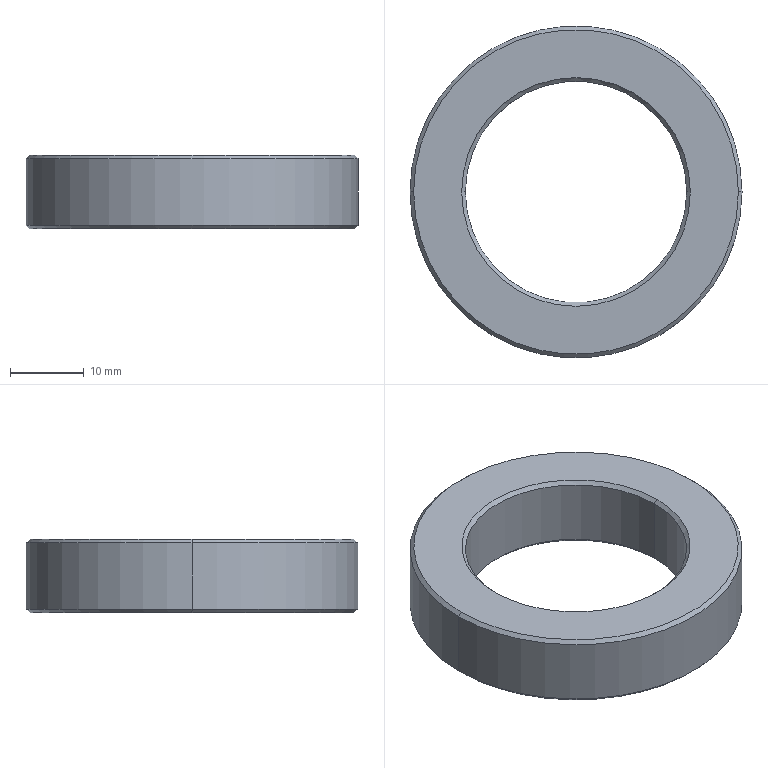Part | SolidWorks | features Chamfer 1, Extrusion 1 | 1 solid | 14 faces | box 45 x 45 x 10 mm | volume 8777 mm3 | cone 8 | cylinder 4 | plane 2 | commonest cylinder face diameters 30 x2 45 x2
STEP:
#1=CARTESIAN_POINT('',(-15.,0.,9.5));
#2=VERTEX_POINT('',#1);
#3=CARTESIAN_POINT('',(15.,0.,9.5));
#4=VERTEX_POINT('',#3);
#5=CARTESIAN_POINT('',(0.,0.,9.5));
#6=DIRECTION('',(0.,0.,1.));
#7=DIRECTION('',(1.,0.,0.));
#8=AXIS2_PLACEMENT_3D('',#5,#6,#7);
#9=CIRCLE('',#8,15.);
#10=EDGE_CURVE('',#2,#4,#9,.T.);
#11=ORIENTED_EDGE('',*,*,#10,.F.);
#12=CARTESIAN_POINT('',(-15.5,0.,10.));
#13=VERTEX_POINT('',#12);
#14=CARTESIAN_POINT('',(-15.,0.,9.5));
#15=DIRECTION('',(-0.7071,0.,0.7071));
#16=VECTOR('',#15,1000.);
#17=LINE('',#14,#16);
#18=EDGE_CURVE('',#2,#13,#17,.T.);
#19=ORIENTED_EDGE('',*,*,#18,.T.);
#20=CARTESIAN_POINT('',(15.5,0.,10.));
#21=VERTEX_POINT('',#20);
#22=CARTESIAN_POINT('',(0.,0.,10.));
#23=DIRECTION('',(0.,0.,-1.));
#24=DIRECTION('',(1.,0.,0.));
#25=AXIS2_PLACEMENT_3D('',#22,#23,#24);
#26=CIRCLE('',#25,15.5);
#27=EDGE_CURVE('',#21,#13,#26,.T.);
#28=ORIENTED_EDGE('',*,*,#27,.F.);
#29=CARTESIAN_POINT('',(15.,0.,9.5));
#30=DIRECTION('',(0.7071,0.,0.7071));
#31=VECTOR('',#30,1000.);
#32=LINE('',#29,#31);
#33=EDGE_CURVE('',#4,#21,#32,.T.);
#34=ORIENTED_EDGE('',*,*,#33,.F.);
#35=EDGE_LOOP('',(#11,#19,#28,#34));
#36=FACE_OUTER_BOUND('',#35,.T.);
#37=CARTESIAN_POINT('',(0.,0.,9.5));
#38=DIRECTION('',(0.,0.,1.));
#39=DIRECTION('',(1.,0.,0.));
#40=AXIS2_PLACEMENT_3D('',#37,#38,#39);
#41=CONICAL_SURFACE('',#40,15.,0.7854);
#42=ADVANCED_FACE('',(#36),#41,.F.);
#43=CARTESIAN_POINT('',(15.,0.,0.5));
#44=VERTEX_POINT('',#43);
#45=CARTESIAN_POINT('',(-15.,0.,0.5));
#46=VERTEX_POINT('',#45);
#47=CARTESIAN_POINT('',(0.,0.,0.5));
#48=DIRECTION('',(0.,0.,-1.));
#49=DIRECTION('',(1.,0.,0.));
#50=AXIS2_PLACEMENT_3D('',#47,#48,#49);
#51=CIRCLE('',#50,15.);
#52=EDGE_CURVE('',#44,#46,#51,.T.);
#53=ORIENTED_EDGE('',*,*,#52,.F.);
#54=CARTESIAN_POINT('',(15.5,0.,0.));
#55=VERTEX_POINT('',#54);
#56=CARTESIAN_POINT('',(15.5,0.,0.));
#57=DIRECTION('',(0.7071,0.,-0.7071));
#58=VECTOR('',#57,1000.);
#59=LINE('',#56,#58);
#60=EDGE_CURVE('',#44,#55,#59,.T.);
#61=ORIENTED_EDGE('',*,*,#60,.T.);
#62=CARTESIAN_POINT('',(-15.5,0.,0.));
#63=VERTEX_POINT('',#62);
#64=CARTESIAN_POINT('',(0.,0.,0.));
#65=DIRECTION('',(0.,0.,1.));
#66=DIRECTION('',(1.,0.,0.));
#67=AXIS2_PLACEMENT_3D('',#64,#65,#66);
#68=CIRCLE('',#67,15.5);
#69=EDGE_CURVE('',#63,#55,#68,.T.);
#70=ORIENTED_EDGE('',*,*,#69,.F.);
#71=CARTESIAN_POINT('',(-15.5,0.,0.));
#72=DIRECTION('',(-0.7071,0.,-0.7071));
#73=VECTOR('',#72,1000.);
#74=LINE('',#71,#73);
#75=EDGE_CURVE('',#46,#63,#74,.T.);
#76=ORIENTED_EDGE('',*,*,#75,.F.);
#77=EDGE_LOOP('',(#53,#61,#70,#76));
#78=FACE_OUTER_BOUND('',#77,.T.);
#79=CARTESIAN_POINT('',(0.,0.,0.));
#80=DIRECTION('',(0.,0.,-1.));
#81=DIRECTION('',(-1.,0.,0.));
#82=AXIS2_PLACEMENT_3D('',#79,#80,#81);
#83=CONICAL_SURFACE('',#82,15.5,0.7854);
#84=ADVANCED_FACE('',(#78),#83,.F.);
#85=CARTESIAN_POINT('',(22.,0.,10.));
#86=VERTEX_POINT('',#85);
#87=CARTESIAN_POINT('',(-22.,0.,10.));
#88=VERTEX_POINT('',#87);
#89=CARTESIAN_POINT('',(0.,0.,10.));
#90=DIRECTION('',(0.,0.,1.));
#91=DIRECTION('',(1.,0.,0.));
#92=AXIS2_PLACEMENT_3D('',#89,#90,#91);
#93=CIRCLE('',#92,22.);
#94=EDGE_CURVE('',#86,#88,#93,.T.);
#95=ORIENTED_EDGE('',*,*,#94,.F.);
#96=CARTESIAN_POINT('',(22.5,0.,9.5));
#97=VERTEX_POINT('',#96);
#98=CARTESIAN_POINT('',(22.,0.,10.));
#99=DIRECTION('',(0.7071,0.,-0.7071));
#100=VECTOR('',#99,1000.);
#101=LINE('',#98,#100);
#102=EDGE_CURVE('',#86,#97,#101,.T.);
#103=ORIENTED_EDGE('',*,*,#102,.T.);
#104=CARTESIAN_POINT('',(-22.5,0.,9.5));
#105=VERTEX_POINT('',#104);
#106=CARTESIAN_POINT('',(0.,0.,9.5));
#107=DIRECTION('',(0.,0.,-1.));
#108=DIRECTION('',(1.,0.,0.));
#109=AXIS2_PLACEMENT_3D('',#106,#107,#108);
#110=CIRCLE('',#109,22.5);
#111=EDGE_CURVE('',#105,#97,#110,.T.);
#112=ORIENTED_EDGE('',*,*,#111,.F.);
#113=CARTESIAN_POINT('',(-22.,0.,10.));
#114=DIRECTION('',(-0.7071,0.,-0.7071));
#115=VECTOR('',#114,1000.);
#116=LINE('',#113,#115);
#117=EDGE_CURVE('',#88,#105,#116,.T.);
#118=ORIENTED_EDGE('',*,*,#117,.F.);
#119=EDGE_LOOP('',(#95,#103,#112,#118));
#120=FACE_OUTER_BOUND('',#119,.T.);
#121=CARTESIAN_POINT('',(0.,0.,10.));
#122=DIRECTION('',(0.,0.,-1.));
#123=DIRECTION('',(-1.,0.,0.));
#124=AXIS2_PLACEMENT_3D('',#121,#122,#123);
#125=CONICAL_SURFACE('',#124,22.,0.7854);
#126=ADVANCED_FACE('',(#120),#125,.T.);
#127=CARTESIAN_POINT('',(-22.,0.,0.));
#128=VERTEX_POINT('',#127);
#129=CARTESIAN_POINT('',(22.,0.,0.));
#130=VERTEX_POINT('',#129);
#131=CARTESIAN_POINT('',(0.,0.,0.));
#132=DIRECTION('',(0.,0.,-1.));
#133=DIRECTION('',(1.,0.,0.));
#134=AXIS2_PLACEMENT_3D('',#131,#132,#133);
#135=CIRCLE('',#134,22.);
#136=EDGE_CURVE('',#128,#130,#135,.T.);
#137=ORIENTED_EDGE('',*,*,#136,.F.);
#138=CARTESIAN_POINT('',(-22.5,0.,0.5));
#139=VERTEX_POINT('',#138);
#140=CARTESIAN_POINT('',(-22.5,0.,0.5));
#141=DIRECTION('',(-0.7071,0.,0.7071));
#142=VECTOR('',#141,1000.);
#143=LINE('',#140,#142);
#144=EDGE_CURVE('',#128,#139,#143,.T.);
#145=ORIENTED_EDGE('',*,*,#144,.T.);
#146=CARTESIAN_POINT('',(22.5,0.,0.5));
#147=VERTEX_POINT('',#146);
#148=CARTESIAN_POINT('',(0.,0.,0.5));
#149=DIRECTION('',(0.,0.,1.));
#150=DIRECTION('',(1.,0.,0.));
#151=AXIS2_PLACEMENT_3D('',#148,#149,#150);
#152=CIRCLE('',#151,22.5);
#153=EDGE_CURVE('',#147,#139,#152,.T.);
#154=ORIENTED_EDGE('',*,*,#153,.F.);
#155=CARTESIAN_POINT('',(22.5,0.,0.5));
#156=DIRECTION('',(0.7071,0.,0.7071));
#157=VECTOR('',#156,1000.);
#158=LINE('',#155,#157);
#159=EDGE_CURVE('',#130,#147,#158,.T.);
#160=ORIENTED_EDGE('',*,*,#159,.F.);
#161=EDGE_LOOP('',(#137,#145,#154,#160));
#162=FACE_OUTER_BOUND('',#161,.T.);
#163=CARTESIAN_POINT('',(0.,0.,0.5));
#164=DIRECTION('',(0.,0.,1.));
#165=DIRECTION('',(1.,0.,0.));
#166=AXIS2_PLACEMENT_3D('',#163,#164,#165);
#167=CONICAL_SURFACE('',#166,22.5,0.7854);
#168=ADVANCED_FACE('',(#162),#167,.T.);
#169=ORIENTED_EDGE('',*,*,#10,.T.);
#170=CARTESIAN_POINT('',(15.,0.,10.));
#171=DIRECTION('',(0.,0.,-1.));
#172=VECTOR('',#171,1000.);
#173=LINE('',#170,#172);
#174=EDGE_CURVE('',#4,#44,#173,.T.);
#175=ORIENTED_EDGE('',*,*,#174,.T.);
#176=ORIENTED_EDGE('',*,*,#52,.T.);
#177=CARTESIAN_POINT('',(-15.,0.,10.));
#178=DIRECTION('',(0.,0.,-1.));
#179=VECTOR('',#178,1000.);
#180=LINE('',#177,#179);
#181=EDGE_CURVE('',#2,#46,#180,.T.);
#182=ORIENTED_EDGE('',*,*,#181,.F.);
#183=EDGE_LOOP('',(#169,#175,#176,#182));
#184=FACE_OUTER_BOUND('',#183,.T.);
#185=CARTESIAN_POINT('',(0.,0.,10.));
#186=DIRECTION('',(0.,0.,-1.));
#187=DIRECTION('',(-1.,0.,0.));
#188=AXIS2_PLACEMENT_3D('',#185,#186,#187);
#189=CYLINDRICAL_SURFACE('',#188,15.);
#190=ADVANCED_FACE('',(#184),#189,.F.);
#191=ORIENTED_EDGE('',*,*,#111,.T.);
#192=CARTESIAN_POINT('',(22.5,0.,10.));
#193=DIRECTION('',(0.,0.,-1.));
#194=VECTOR('',#193,1000.);
#195=LINE('',#192,#194);
#196=EDGE_CURVE('',#97,#147,#195,.T.);
#197=ORIENTED_EDGE('',*,*,#196,.T.);
#198=ORIENTED_EDGE('',*,*,#153,.T.);
#199=CARTESIAN_POINT('',(-22.5,0.,10.));
#200=DIRECTION('',(0.,0.,-1.));
#201=VECTOR('',#200,1000.);
#202=LINE('',#199,#201);
#203=EDGE_CURVE('',#105,#139,#202,.T.);
#204=ORIENTED_EDGE('',*,*,#203,.F.);
#205=EDGE_LOOP('',(#191,#197,#198,#204));
#206=FACE_OUTER_BOUND('',#205,.T.);
#207=CARTESIAN_POINT('',(0.,0.,10.));
#208=DIRECTION('',(0.,0.,-1.));
#209=DIRECTION('',(-1.,0.,0.));
#210=AXIS2_PLACEMENT_3D('',#207,#208,#209);
#211=CYLINDRICAL_SURFACE('',#210,22.5);
#212=ADVANCED_FACE('',(#206),#211,.T.);
#213=CARTESIAN_POINT('',(0.,0.,10.));
#214=DIRECTION('',(0.,0.,1.));
#215=DIRECTION('',(1.,0.,0.));
#216=AXIS2_PLACEMENT_3D('',#213,#214,#215);
#217=CIRCLE('',#216,22.);
#218=EDGE_CURVE('',#88,#86,#217,.T.);
#219=ORIENTED_EDGE('',*,*,#218,.T.);
#220=ORIENTED_EDGE('',*,*,#94,.T.);
#221=EDGE_LOOP('',(#219,#220));
#222=FACE_OUTER_BOUND('',#221,.T.);
#223=ORIENTED_EDGE('',*,*,#27,.T.);
#224=CARTESIAN_POINT('',(0.,0.,10.));
#225=DIRECTION('',(0.,0.,-1.));
#226=DIRECTION('',(1.,0.,0.));
#227=AXIS2_PLACEMENT_3D('',#224,#225,#226);
#228=CIRCLE('',#227,15.5);
#229=EDGE_CURVE('',#13,#21,#228,.T.);
#230=ORIENTED_EDGE('',*,*,#229,.T.);
#231=EDGE_LOOP('',(#223,#230));
#232=FACE_BOUND('',#231,.T.);
#233=CARTESIAN_POINT('',(0.,0.,10.));
#234=DIRECTION('',(0.,0.,1.));
#235=DIRECTION('',(1.,0.,0.));
#236=AXIS2_PLACEMENT_3D('',#233,#234,#235);
#237=PLANE('',#236);
#238=ADVANCED_FACE('',(#222,#232),#237,.T.);
#239=CARTESIAN_POINT('',(0.,0.,0.));
#240=DIRECTION('',(0.,0.,-1.));
#241=DIRECTION('',(1.,0.,0.));
#242=AXIS2_PLACEMENT_3D('',#239,#240,#241);
#243=CIRCLE('',#242,22.);
#244=EDGE_CURVE('',#130,#128,#243,.T.);
#245=ORIENTED_EDGE('',*,*,#244,.T.);
#246=ORIENTED_EDGE('',*,*,#136,.T.);
#247=EDGE_LOOP('',(#245,#246));
#248=FACE_OUTER_BOUND('',#247,.T.);
#249=ORIENTED_EDGE('',*,*,#69,.T.);
#250=CARTESIAN_POINT('',(0.,0.,0.));
#251=DIRECTION('',(0.,0.,1.));
#252=DIRECTION('',(1.,0.,0.));
#253=AXIS2_PLACEMENT_3D('',#250,#251,#252);
#254=CIRCLE('',#253,15.5);
#255=EDGE_CURVE('',#55,#63,#254,.T.);
#256=ORIENTED_EDGE('',*,*,#255,.T.);
#257=EDGE_LOOP('',(#249,#256));
#258=FACE_BOUND('',#257,.T.);
#259=CARTESIAN_POINT('',(0.,0.,0.));
#260=DIRECTION('',(0.,0.,1.));
#261=DIRECTION('',(1.,0.,0.));
#262=AXIS2_PLACEMENT_3D('',#259,#260,#261);
#263=PLANE('',#262);
#264=ADVANCED_FACE('',(#248,#258),#263,.F.);
#265=ORIENTED_EDGE('',*,*,#196,.F.);
#266=CARTESIAN_POINT('',(0.,0.,9.5));
#267=DIRECTION('',(0.,0.,-1.));
#268=DIRECTION('',(1.,0.,0.));
#269=AXIS2_PLACEMENT_3D('',#266,#267,#268);
#270=CIRCLE('',#269,22.5);
#271=EDGE_CURVE('',#97,#105,#270,.T.);
#272=ORIENTED_EDGE('',*,*,#271,.T.);
#273=ORIENTED_EDGE('',*,*,#203,.T.);
#274=CARTESIAN_POINT('',(0.,0.,0.5));
#275=DIRECTION('',(0.,0.,1.));
#276=DIRECTION('',(1.,0.,0.));
#277=AXIS2_PLACEMENT_3D('',#274,#275,#276);
#278=CIRCLE('',#277,22.5);
#279=EDGE_CURVE('',#139,#147,#278,.T.);
#280=ORIENTED_EDGE('',*,*,#279,.T.);
#281=EDGE_LOOP('',(#265,#272,#273,#280));
#282=FACE_OUTER_BOUND('',#281,.T.);
#283=CARTESIAN_POINT('',(0.,0.,10.));
#284=DIRECTION('',(0.,0.,-1.));
#285=DIRECTION('',(-1.,0.,0.));
#286=AXIS2_PLACEMENT_3D('',#283,#284,#285);
#287=CYLINDRICAL_SURFACE('',#286,22.5);
#288=ADVANCED_FACE('',(#282),#287,.T.);
#289=ORIENTED_EDGE('',*,*,#174,.F.);
#290=CARTESIAN_POINT('',(0.,0.,9.5));
#291=DIRECTION('',(0.,0.,1.));
#292=DIRECTION('',(1.,0.,0.));
#293=AXIS2_PLACEMENT_3D('',#290,#291,#292);
#294=CIRCLE('',#293,15.);
#295=EDGE_CURVE('',#4,#2,#294,.T.);
#296=ORIENTED_EDGE('',*,*,#295,.T.);
#297=ORIENTED_EDGE('',*,*,#181,.T.);
#298=CARTESIAN_POINT('',(0.,0.,0.5));
#299=DIRECTION('',(0.,0.,-1.));
#300=DIRECTION('',(1.,0.,0.));
#301=AXIS2_PLACEMENT_3D('',#298,#299,#300);
#302=CIRCLE('',#301,15.);
#303=EDGE_CURVE('',#46,#44,#302,.T.);
#304=ORIENTED_EDGE('',*,*,#303,.T.);
#305=EDGE_LOOP('',(#289,#296,#297,#304));
#306=FACE_OUTER_BOUND('',#305,.T.);
#307=CARTESIAN_POINT('',(0.,0.,10.));
#308=DIRECTION('',(0.,0.,-1.));
#309=DIRECTION('',(-1.,0.,0.));
#310=AXIS2_PLACEMENT_3D('',#307,#308,#309);
#311=CYLINDRICAL_SURFACE('',#310,15.);
#312=ADVANCED_FACE('',(#306),#311,.F.);
#313=ORIENTED_EDGE('',*,*,#144,.F.);
#314=ORIENTED_EDGE('',*,*,#244,.F.);
#315=ORIENTED_EDGE('',*,*,#159,.T.);
#316=ORIENTED_EDGE('',*,*,#279,.F.);
#317=EDGE_LOOP('',(#313,#314,#315,#316));
#318=FACE_OUTER_BOUND('',#317,.T.);
#319=CARTESIAN_POINT('',(0.,0.,0.5));
#320=DIRECTION('',(0.,0.,1.));
#321=DIRECTION('',(1.,0.,0.));
#322=AXIS2_PLACEMENT_3D('',#319,#320,#321);
#323=CONICAL_SURFACE('',#322,22.5,0.7854);
#324=ADVANCED_FACE('',(#318),#323,.T.);
#325=ORIENTED_EDGE('',*,*,#102,.F.);
#326=ORIENTED_EDGE('',*,*,#218,.F.);
#327=ORIENTED_EDGE('',*,*,#117,.T.);
#328=ORIENTED_EDGE('',*,*,#271,.F.);
#329=EDGE_LOOP('',(#325,#326,#327,#328));
#330=FACE_OUTER_BOUND('',#329,.T.);
#331=CARTESIAN_POINT('',(0.,0.,10.));
#332=DIRECTION('',(0.,0.,-1.));
#333=DIRECTION('',(-1.,0.,0.));
#334=AXIS2_PLACEMENT_3D('',#331,#332,#333);
#335=CONICAL_SURFACE('',#334,22.,0.7854);
#336=ADVANCED_FACE('',(#330),#335,.T.);
#337=ORIENTED_EDGE('',*,*,#60,.F.);
#338=ORIENTED_EDGE('',*,*,#303,.F.);
#339=ORIENTED_EDGE('',*,*,#75,.T.);
#340=ORIENTED_EDGE('',*,*,#255,.F.);
#341=EDGE_LOOP('',(#337,#338,#339,#340));
#342=FACE_OUTER_BOUND('',#341,.T.);
#343=CARTESIAN_POINT('',(0.,0.,0.));
#344=DIRECTION('',(0.,0.,-1.));
#345=DIRECTION('',(-1.,0.,0.));
#346=AXIS2_PLACEMENT_3D('',#343,#344,#345);
#347=CONICAL_SURFACE('',#346,15.5,0.7854);
#348=ADVANCED_FACE('',(#342),#347,.F.);
#349=ORIENTED_EDGE('',*,*,#18,.F.);
#350=ORIENTED_EDGE('',*,*,#295,.F.);
#351=ORIENTED_EDGE('',*,*,#33,.T.);
#352=ORIENTED_EDGE('',*,*,#229,.F.);
#353=EDGE_LOOP('',(#349,#350,#351,#352));
#354=FACE_OUTER_BOUND('',#353,.T.);
#355=CARTESIAN_POINT('',(0.,0.,9.5));
#356=DIRECTION('',(0.,0.,1.));
#357=DIRECTION('',(1.,0.,0.));
#358=AXIS2_PLACEMENT_3D('',#355,#356,#357);
#359=CONICAL_SURFACE('',#358,15.,0.7854);
#360=ADVANCED_FACE('',(#354),#359,.F.);
#361=CLOSED_SHELL('',(#42,#84,#126,#168,#190,#212,#238,#264,#288,#312,#324,#336,#348,#360));
#362=MANIFOLD_SOLID_BREP('',#361);
#363=CARTESIAN_POINT('',(0.,0.,0.));
#364=DIRECTION('',(0.,0.,1.));
#365=DIRECTION('',(1.,0.,0.));
#366=AXIS2_PLACEMENT_3D('',#363,#364,#365);
#367=(LENGTH_UNIT()NAMED_UNIT(*)SI_UNIT(.MILLI.,.METRE.));
#368=UNCERTAINTY_MEASURE_WITH_UNIT(LENGTH_MEASURE(0.00001),#367,'','');
#369=(NAMED_UNIT(*)PLANE_ANGLE_UNIT()SI_UNIT($,.RADIAN.));
#370=(NAMED_UNIT(*)SI_UNIT($,.STERADIAN.)SOLID_ANGLE_UNIT());
#371=(GEOMETRIC_REPRESENTATION_CONTEXT(3)GLOBAL_UNCERTAINTY_ASSIGNED_CONTEXT((#368))GLOBAL_UNIT_ASSIGNED_CONTEXT((#367,#369,#370))REPRESENTATION_CONTEXT('',''));
#372=ADVANCED_BREP_SHAPE_REPRESENTATION('',(#362,#366),#371);